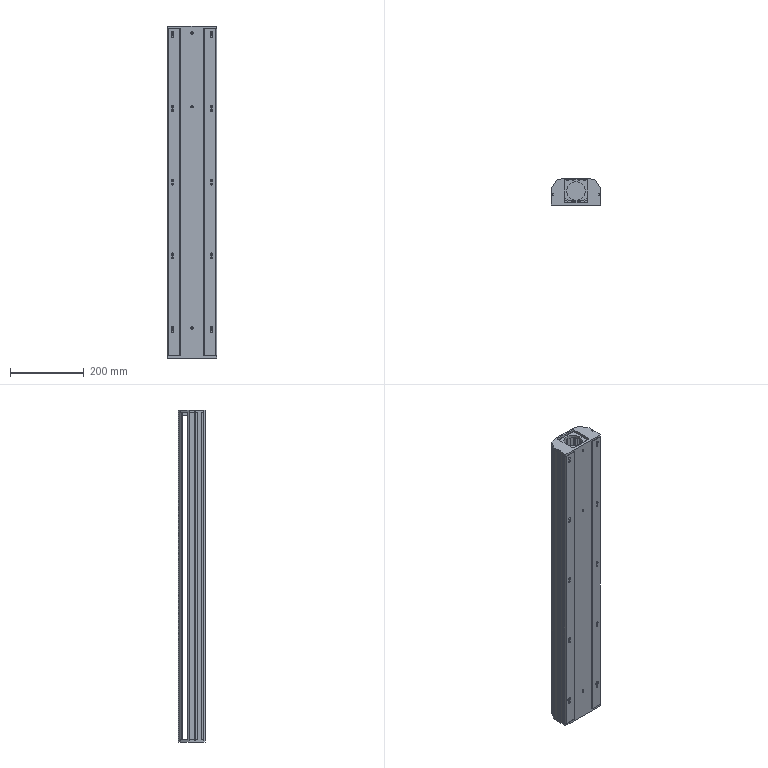Part | STEP file | 2 solids | 473 faces | box 135 x 74.2 x 900.5 mm | volume 2232151 mm3 | cylinder 245 | plane 228 | commonest cylinder face diameters 0.6 x84 6 x24 11 x24 5.2 x20 7 x20 2 x18